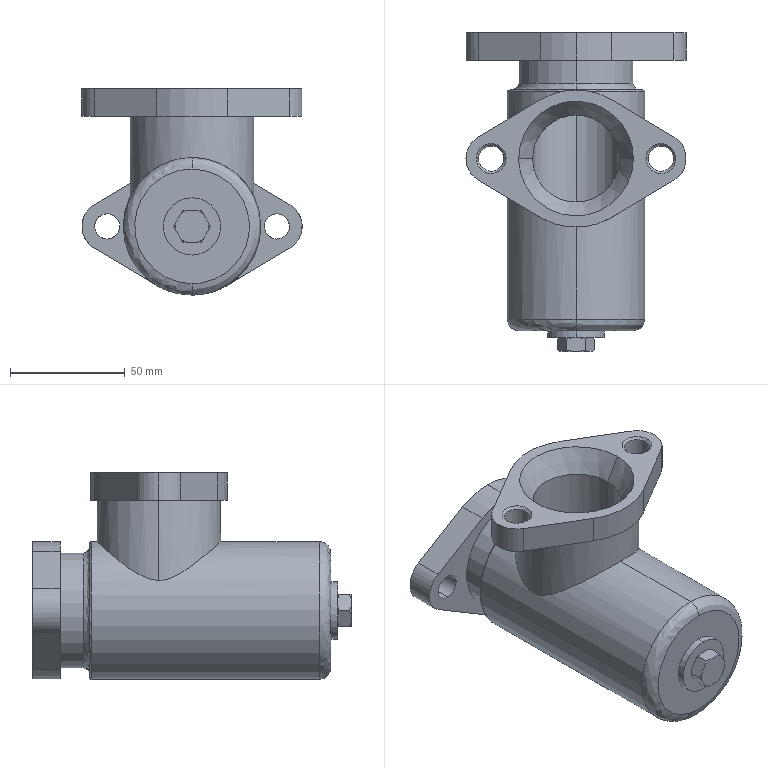Part | SolidWorks | features BaseBody 2 | 2 solids | 107 faces | box 96 x 139 x 90 mm | volume 267459 mm3 | cylinder 51 | plane 25 | cone 21 | spline 8 | torus 2 | commonest cylinder face diameters 9 x21 11 x8 60 x7 22 x5 38 x4 25 x2